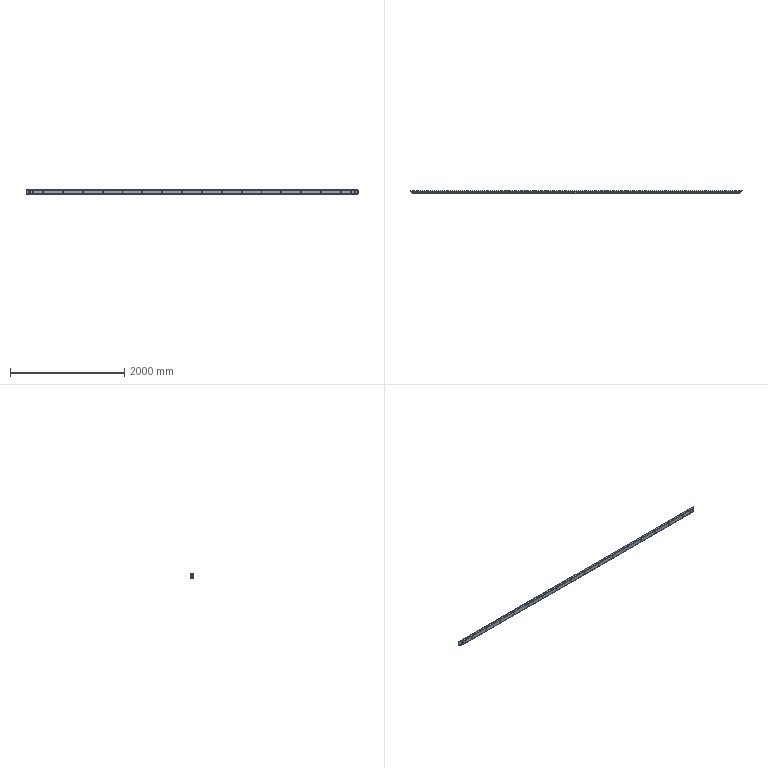Part | STEP file | SN10_003_008-01_TUBO_RETANGULAR | 1 solid | 98 faces | box 5820 x 40 x 80 mm | volume 3744159 mm3 | cylinder 88 | plane 10 | commonest cylinder face diameters 20 x80 6 x4 12 x4